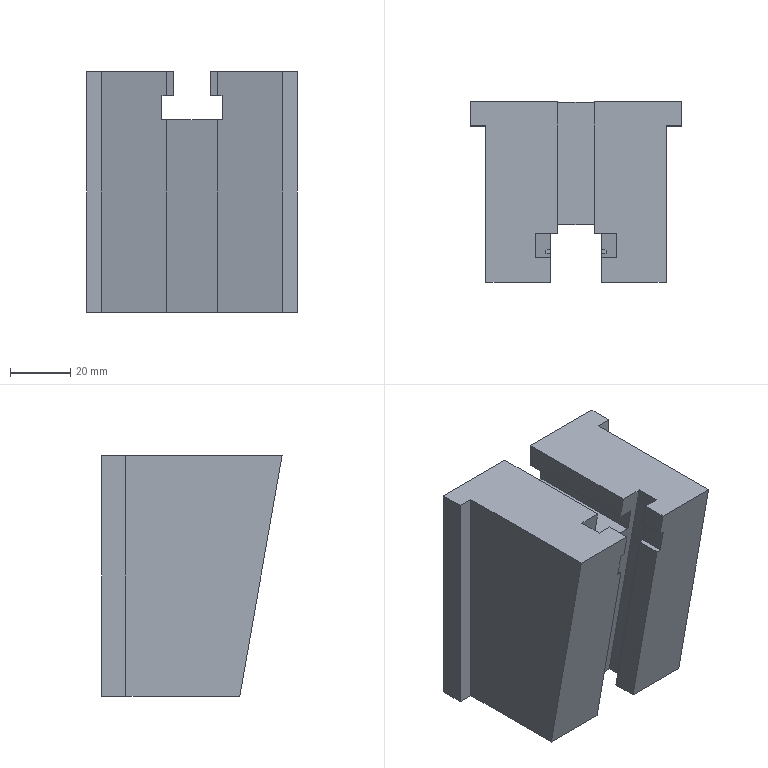Part | STEP file | solid 143 | 1 solid | 34 faces | box 70 x 60 x 80 mm | volume 220295 mm3 | plane 34